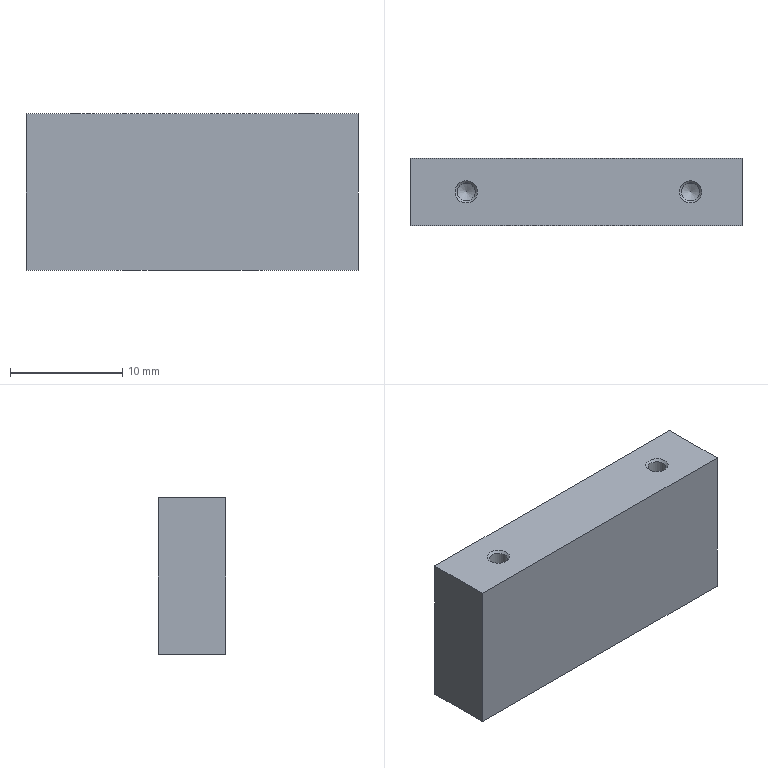Part | STEP file | Final stage amplifier press block | 1 solid | 18 faces | box 29.61 x 6 x 14 mm | volume 2437 mm3 | cone 8 | plane 6 | cylinder 4 | commonest cylinder face diameters 1.6 x4
STEP:
#1=CARTESIAN_POINT('',(0.,0.,0.));
#2=DIRECTION('',(0.,0.,1.));
#3=DIRECTION('',(1.,0.,0.));
#4=AXIS2_PLACEMENT_3D('',#1,#2,#3);
#5=CARTESIAN_POINT('',(-8.334,90.75,188.564));
#6=VERTEX_POINT('',#5);
#7=CARTESIAN_POINT('',(-8.334,84.75,188.564));
#8=VERTEX_POINT('',#7);
#9=CARTESIAN_POINT('',(-8.334,90.75,188.564));
#10=DIRECTION('',(0.,-1.,0.));
#11=VECTOR('',#10,1.);
#12=LINE('',#9,#11);
#13=CARTESIAN_POINT('',(-8.334,90.75,202.564));
#14=DIRECTION('',(1.,0.,0.));
#15=DIRECTION('',(0.,0.,-1.));
#16=AXIS2_PLACEMENT_3D('',#13,#14,#15);
#17=PLANE('',#16);
#18=CARTESIAN_POINT('',(14.,0.));
#19=DIRECTION('',(0.,-1.));
#20=VECTOR('',#19,1.);
#21=LINE('',#18,#20);
#22=(GEOMETRIC_REPRESENTATION_CONTEXT(2)PARAMETRIC_REPRESENTATION_CONTEXT()REPRESENTATION_CONTEXT('',''));
#23=DEFINITIONAL_REPRESENTATION('',(#21),#22);
#24=PCURVE('',#17,#23);
#25=CARTESIAN_POINT('',(0.,0.,188.564));
#26=DIRECTION('',(0.,0.,1.));
#27=DIRECTION('',(1.,0.,0.));
#28=AXIS2_PLACEMENT_3D('',#25,#26,#27);
#29=PLANE('',#28);
#30=CARTESIAN_POINT('',(-8.334,90.75));
#31=DIRECTION('',(0.,-1.));
#32=VECTOR('',#31,1.);
#33=LINE('',#30,#32);
#34=(GEOMETRIC_REPRESENTATION_CONTEXT(2)PARAMETRIC_REPRESENTATION_CONTEXT()REPRESENTATION_CONTEXT('',''));
#35=DEFINITIONAL_REPRESENTATION('',(#33),#34);
#36=PCURVE('',#29,#35);
#37=SURFACE_CURVE('',#12,(#24,#36),.PCURVE_S1.);
#38=EDGE_CURVE('',#6,#8,#37,.T.);
#39=ORIENTED_EDGE('',*,*,#38,.T.);
#40=CARTESIAN_POINT('',(-8.334,84.75,202.564));
#41=VERTEX_POINT('',#40);
#42=CARTESIAN_POINT('',(-8.334,84.75,202.564));
#43=DIRECTION('',(0.,0.,-1.));
#44=VECTOR('',#43,1.);
#45=LINE('',#42,#44);
#46=CARTESIAN_POINT('',(0.,-6.));
#47=DIRECTION('',(1.,0.));
#48=VECTOR('',#47,1.);
#49=LINE('',#46,#48);
#50=(GEOMETRIC_REPRESENTATION_CONTEXT(2)PARAMETRIC_REPRESENTATION_CONTEXT()REPRESENTATION_CONTEXT('',''));
#51=DEFINITIONAL_REPRESENTATION('',(#49),#50);
#52=PCURVE('',#17,#51);
#53=CARTESIAN_POINT('',(-8.334,84.75,202.564));
#54=DIRECTION('',(0.,1.,0.));
#55=DIRECTION('',(0.,0.,1.));
#56=AXIS2_PLACEMENT_3D('',#53,#54,#55);
#57=PLANE('',#56);
#58=CARTESIAN_POINT('',(0.,0.));
#59=DIRECTION('',(-1.,0.));
#60=VECTOR('',#59,1.);
#61=LINE('',#58,#60);
#62=(GEOMETRIC_REPRESENTATION_CONTEXT(2)PARAMETRIC_REPRESENTATION_CONTEXT()REPRESENTATION_CONTEXT('',''));
#63=DEFINITIONAL_REPRESENTATION('',(#61),#62);
#64=PCURVE('',#57,#63);
#65=SURFACE_CURVE('',#45,(#52,#64),.PCURVE_S1.);
#66=EDGE_CURVE('',#41,#8,#65,.T.);
#67=ORIENTED_EDGE('',*,*,#66,.F.);
#68=CARTESIAN_POINT('',(-8.334,90.75,202.564));
#69=VERTEX_POINT('',#68);
#70=CARTESIAN_POINT('',(-8.334,90.75,202.564));
#71=DIRECTION('',(0.,-1.,0.));
#72=VECTOR('',#71,1.);
#73=LINE('',#70,#72);
#74=CARTESIAN_POINT('',(0.,0.));
#75=DIRECTION('',(0.,-1.));
#76=VECTOR('',#75,1.);
#77=LINE('',#74,#76);
#78=(GEOMETRIC_REPRESENTATION_CONTEXT(2)PARAMETRIC_REPRESENTATION_CONTEXT()REPRESENTATION_CONTEXT('',''));
#79=DEFINITIONAL_REPRESENTATION('',(#77),#78);
#80=PCURVE('',#17,#79);
#81=CARTESIAN_POINT('',(0.,0.,202.564));
#82=DIRECTION('',(0.,0.,1.));
#83=DIRECTION('',(1.,0.,0.));
#84=AXIS2_PLACEMENT_3D('',#81,#82,#83);
#85=PLANE('',#84);
#86=CARTESIAN_POINT('',(-8.334,90.75));
#87=DIRECTION('',(0.,-1.));
#88=VECTOR('',#87,1.);
#89=LINE('',#86,#88);
#90=(GEOMETRIC_REPRESENTATION_CONTEXT(2)PARAMETRIC_REPRESENTATION_CONTEXT()REPRESENTATION_CONTEXT('',''));
#91=DEFINITIONAL_REPRESENTATION('',(#89),#90);
#92=PCURVE('',#85,#91);
#93=SURFACE_CURVE('',#73,(#80,#92),.PCURVE_S1.);
#94=EDGE_CURVE('',#69,#41,#93,.T.);
#95=ORIENTED_EDGE('',*,*,#94,.F.);
#96=CARTESIAN_POINT('',(-8.334,90.75,202.564));
#97=DIRECTION('',(0.,0.,-1.));
#98=VECTOR('',#97,1.);
#99=LINE('',#96,#98);
#100=CARTESIAN_POINT('',(0.,0.));
#101=DIRECTION('',(1.,0.));
#102=VECTOR('',#101,1.);
#103=LINE('',#100,#102);
#104=(GEOMETRIC_REPRESENTATION_CONTEXT(2)PARAMETRIC_REPRESENTATION_CONTEXT()REPRESENTATION_CONTEXT('',''));
#105=DEFINITIONAL_REPRESENTATION('',(#103),#104);
#106=PCURVE('',#17,#105);
#107=CARTESIAN_POINT('',(21.276,90.75,202.564));
#108=DIRECTION('',(0.,-1.,0.));
#109=DIRECTION('',(0.,0.,-1.));
#110=AXIS2_PLACEMENT_3D('',#107,#108,#109);
#111=PLANE('',#110);
#112=CARTESIAN_POINT('',(0.,-29.61));
#113=DIRECTION('',(1.,0.));
#114=VECTOR('',#113,1.);
#115=LINE('',#112,#114);
#116=(GEOMETRIC_REPRESENTATION_CONTEXT(2)PARAMETRIC_REPRESENTATION_CONTEXT()REPRESENTATION_CONTEXT('',''));
#117=DEFINITIONAL_REPRESENTATION('',(#115),#116);
#118=PCURVE('',#111,#117);
#119=SURFACE_CURVE('',#99,(#106,#118),.PCURVE_S1.);
#120=EDGE_CURVE('',#69,#6,#119,.T.);
#121=ORIENTED_EDGE('',*,*,#120,.T.);
#122=EDGE_LOOP('',(#39,#67,#95,#121));
#123=FACE_BOUND('',#122,.T.);
#124=ADVANCED_FACE('',(#123),#17,.F.);
#125=CARTESIAN_POINT('',(21.276,84.75,188.564));
#126=VERTEX_POINT('',#125);
#127=CARTESIAN_POINT('',(-8.334,84.75,188.564));
#128=DIRECTION('',(1.,0.,0.));
#129=VECTOR('',#128,1.);
#130=LINE('',#127,#129);
#131=CARTESIAN_POINT('',(-14.,0.));
#132=DIRECTION('',(0.,1.));
#133=VECTOR('',#132,1.);
#134=LINE('',#131,#133);
#135=(GEOMETRIC_REPRESENTATION_CONTEXT(2)PARAMETRIC_REPRESENTATION_CONTEXT()REPRESENTATION_CONTEXT('',''));
#136=DEFINITIONAL_REPRESENTATION('',(#134),#135);
#137=PCURVE('',#57,#136);
#138=CARTESIAN_POINT('',(-8.334,84.75));
#139=DIRECTION('',(1.,0.));
#140=VECTOR('',#139,1.);
#141=LINE('',#138,#140);
#142=(GEOMETRIC_REPRESENTATION_CONTEXT(2)PARAMETRIC_REPRESENTATION_CONTEXT()REPRESENTATION_CONTEXT('',''));
#143=DEFINITIONAL_REPRESENTATION('',(#141),#142);
#144=PCURVE('',#29,#143);
#145=SURFACE_CURVE('',#130,(#137,#144),.PCURVE_S1.);
#146=EDGE_CURVE('',#8,#126,#145,.T.);
#147=ORIENTED_EDGE('',*,*,#146,.T.);
#148=CARTESIAN_POINT('',(21.276,84.75,202.564));
#149=VERTEX_POINT('',#148);
#150=CARTESIAN_POINT('',(21.276,84.75,202.564));
#151=DIRECTION('',(0.,0.,-1.));
#152=VECTOR('',#151,1.);
#153=LINE('',#150,#152);
#154=CARTESIAN_POINT('',(0.,29.61));
#155=DIRECTION('',(-1.,0.));
#156=VECTOR('',#155,1.);
#157=LINE('',#154,#156);
#158=(GEOMETRIC_REPRESENTATION_CONTEXT(2)PARAMETRIC_REPRESENTATION_CONTEXT()REPRESENTATION_CONTEXT('',''));
#159=DEFINITIONAL_REPRESENTATION('',(#157),#158);
#160=PCURVE('',#57,#159);
#161=CARTESIAN_POINT('',(21.276,84.75,202.564));
#162=DIRECTION('',(-1.,0.,0.));
#163=DIRECTION('',(0.,0.,1.));
#164=AXIS2_PLACEMENT_3D('',#161,#162,#163);
#165=PLANE('',#164);
#166=CARTESIAN_POINT('',(0.,0.));
#167=DIRECTION('',(-1.,0.));
#168=VECTOR('',#167,1.);
#169=LINE('',#166,#168);
#170=(GEOMETRIC_REPRESENTATION_CONTEXT(2)PARAMETRIC_REPRESENTATION_CONTEXT()REPRESENTATION_CONTEXT('',''));
#171=DEFINITIONAL_REPRESENTATION('',(#169),#170);
#172=PCURVE('',#165,#171);
#173=SURFACE_CURVE('',#153,(#160,#172),.PCURVE_S1.);
#174=EDGE_CURVE('',#149,#126,#173,.T.);
#175=ORIENTED_EDGE('',*,*,#174,.F.);
#176=CARTESIAN_POINT('',(-8.334,84.75,202.564));
#177=DIRECTION('',(1.,0.,0.));
#178=VECTOR('',#177,1.);
#179=LINE('',#176,#178);
#180=CARTESIAN_POINT('',(0.,0.));
#181=DIRECTION('',(0.,1.));
#182=VECTOR('',#181,1.);
#183=LINE('',#180,#182);
#184=(GEOMETRIC_REPRESENTATION_CONTEXT(2)PARAMETRIC_REPRESENTATION_CONTEXT()REPRESENTATION_CONTEXT('',''));
#185=DEFINITIONAL_REPRESENTATION('',(#183),#184);
#186=PCURVE('',#57,#185);
#187=CARTESIAN_POINT('',(-8.334,84.75));
#188=DIRECTION('',(1.,0.));
#189=VECTOR('',#188,1.);
#190=LINE('',#187,#189);
#191=(GEOMETRIC_REPRESENTATION_CONTEXT(2)PARAMETRIC_REPRESENTATION_CONTEXT()REPRESENTATION_CONTEXT('',''));
#192=DEFINITIONAL_REPRESENTATION('',(#190),#191);
#193=PCURVE('',#85,#192);
#194=SURFACE_CURVE('',#179,(#186,#193),.PCURVE_S1.);
#195=EDGE_CURVE('',#41,#149,#194,.T.);
#196=ORIENTED_EDGE('',*,*,#195,.F.);
#197=ORIENTED_EDGE('',*,*,#66,.T.);
#198=EDGE_LOOP('',(#147,#175,#196,#197));
#199=FACE_BOUND('',#198,.T.);
#200=ADVANCED_FACE('',(#199),#57,.F.);
#201=CARTESIAN_POINT('',(21.276,90.75,188.564));
#202=VERTEX_POINT('',#201);
#203=CARTESIAN_POINT('',(21.276,84.75,188.564));
#204=DIRECTION('',(0.,1.,0.));
#205=VECTOR('',#204,1.);
#206=LINE('',#203,#205);
#207=CARTESIAN_POINT('',(-14.,0.));
#208=DIRECTION('',(0.,1.));
#209=VECTOR('',#208,1.);
#210=LINE('',#207,#209);
#211=(GEOMETRIC_REPRESENTATION_CONTEXT(2)PARAMETRIC_REPRESENTATION_CONTEXT()REPRESENTATION_CONTEXT('',''));
#212=DEFINITIONAL_REPRESENTATION('',(#210),#211);
#213=PCURVE('',#165,#212);
#214=CARTESIAN_POINT('',(21.276,84.75));
#215=DIRECTION('',(0.,1.));
#216=VECTOR('',#215,1.);
#217=LINE('',#214,#216);
#218=(GEOMETRIC_REPRESENTATION_CONTEXT(2)PARAMETRIC_REPRESENTATION_CONTEXT()REPRESENTATION_CONTEXT('',''));
#219=DEFINITIONAL_REPRESENTATION('',(#217),#218);
#220=PCURVE('',#29,#219);
#221=SURFACE_CURVE('',#206,(#213,#220),.PCURVE_S1.);
#222=EDGE_CURVE('',#126,#202,#221,.T.);
#223=ORIENTED_EDGE('',*,*,#222,.T.);
#224=CARTESIAN_POINT('',(21.276,90.75,202.564));
#225=VERTEX_POINT('',#224);
#226=CARTESIAN_POINT('',(21.276,90.75,202.564));
#227=DIRECTION('',(0.,0.,-1.));
#228=VECTOR('',#227,1.);
#229=LINE('',#226,#228);
#230=CARTESIAN_POINT('',(0.,6.));
#231=DIRECTION('',(-1.,0.));
#232=VECTOR('',#231,1.);
#233=LINE('',#230,#232);
#234=(GEOMETRIC_REPRESENTATION_CONTEXT(2)PARAMETRIC_REPRESENTATION_CONTEXT()REPRESENTATION_CONTEXT('',''));
#235=DEFINITIONAL_REPRESENTATION('',(#233),#234);
#236=PCURVE('',#165,#235);
#237=CARTESIAN_POINT('',(0.,0.));
#238=DIRECTION('',(1.,0.));
#239=VECTOR('',#238,1.);
#240=LINE('',#237,#239);
#241=(GEOMETRIC_REPRESENTATION_CONTEXT(2)PARAMETRIC_REPRESENTATION_CONTEXT()REPRESENTATION_CONTEXT('',''));
#242=DEFINITIONAL_REPRESENTATION('',(#240),#241);
#243=PCURVE('',#111,#242);
#244=SURFACE_CURVE('',#229,(#236,#243),.PCURVE_S1.);
#245=EDGE_CURVE('',#225,#202,#244,.T.);
#246=ORIENTED_EDGE('',*,*,#245,.F.);
#247=CARTESIAN_POINT('',(21.276,84.75,202.564));
#248=DIRECTION('',(0.,1.,0.));
#249=VECTOR('',#248,1.);
#250=LINE('',#247,#249);
#251=CARTESIAN_POINT('',(0.,0.));
#252=DIRECTION('',(0.,1.));
#253=VECTOR('',#252,1.);
#254=LINE('',#251,#253);
#255=(GEOMETRIC_REPRESENTATION_CONTEXT(2)PARAMETRIC_REPRESENTATION_CONTEXT()REPRESENTATION_CONTEXT('',''));
#256=DEFINITIONAL_REPRESENTATION('',(#254),#255);
#257=PCURVE('',#165,#256);
#258=CARTESIAN_POINT('',(21.276,84.75));
#259=DIRECTION('',(0.,1.));
#260=VECTOR('',#259,1.);
#261=LINE('',#258,#260);
#262=(GEOMETRIC_REPRESENTATION_CONTEXT(2)PARAMETRIC_REPRESENTATION_CONTEXT()REPRESENTATION_CONTEXT('',''));
#263=DEFINITIONAL_REPRESENTATION('',(#261),#262);
#264=PCURVE('',#85,#263);
#265=SURFACE_CURVE('',#250,(#257,#264),.PCURVE_S1.);
#266=EDGE_CURVE('',#149,#225,#265,.T.);
#267=ORIENTED_EDGE('',*,*,#266,.F.);
#268=ORIENTED_EDGE('',*,*,#174,.T.);
#269=EDGE_LOOP('',(#223,#246,#267,#268));
#270=FACE_BOUND('',#269,.T.);
#271=ADVANCED_FACE('',(#270),#165,.F.);
#272=CARTESIAN_POINT('',(21.276,90.75,188.564));
#273=DIRECTION('',(-1.,0.,0.));
#274=VECTOR('',#273,1.);
#275=LINE('',#272,#274);
#276=CARTESIAN_POINT('',(14.,0.));
#277=DIRECTION('',(0.,-1.));
#278=VECTOR('',#277,1.);
#279=LINE('',#276,#278);
#280=(GEOMETRIC_REPRESENTATION_CONTEXT(2)PARAMETRIC_REPRESENTATION_CONTEXT()REPRESENTATION_CONTEXT('',''));
#281=DEFINITIONAL_REPRESENTATION('',(#279),#280);
#282=PCURVE('',#111,#281);
#283=CARTESIAN_POINT('',(21.276,90.75));
#284=DIRECTION('',(-1.,0.));
#285=VECTOR('',#284,1.);
#286=LINE('',#283,#285);
#287=(GEOMETRIC_REPRESENTATION_CONTEXT(2)PARAMETRIC_REPRESENTATION_CONTEXT()REPRESENTATION_CONTEXT('',''));
#288=DEFINITIONAL_REPRESENTATION('',(#286),#287);
#289=PCURVE('',#29,#288);
#290=SURFACE_CURVE('',#275,(#282,#289),.PCURVE_S1.);
#291=EDGE_CURVE('',#202,#6,#290,.T.);
#292=ORIENTED_EDGE('',*,*,#291,.T.);
#293=ORIENTED_EDGE('',*,*,#120,.F.);
#294=CARTESIAN_POINT('',(21.276,90.75,202.564));
#295=DIRECTION('',(-1.,0.,0.));
#296=VECTOR('',#295,1.);
#297=LINE('',#294,#296);
#298=CARTESIAN_POINT('',(0.,0.));
#299=DIRECTION('',(0.,-1.));
#300=VECTOR('',#299,1.);
#301=LINE('',#298,#300);
#302=(GEOMETRIC_REPRESENTATION_CONTEXT(2)PARAMETRIC_REPRESENTATION_CONTEXT()REPRESENTATION_CONTEXT('',''));
#303=DEFINITIONAL_REPRESENTATION('',(#301),#302);
#304=PCURVE('',#111,#303);
#305=CARTESIAN_POINT('',(21.276,90.75));
#306=DIRECTION('',(-1.,0.));
#307=VECTOR('',#306,1.);
#308=LINE('',#305,#307);
#309=(GEOMETRIC_REPRESENTATION_CONTEXT(2)PARAMETRIC_REPRESENTATION_CONTEXT()REPRESENTATION_CONTEXT('',''));
#310=DEFINITIONAL_REPRESENTATION('',(#308),#309);
#311=PCURVE('',#85,#310);
#312=SURFACE_CURVE('',#297,(#304,#311),.PCURVE_S1.);
#313=EDGE_CURVE('',#225,#69,#312,.T.);
#314=ORIENTED_EDGE('',*,*,#313,.F.);
#315=ORIENTED_EDGE('',*,*,#245,.T.);
#316=EDGE_LOOP('',(#292,#293,#314,#315));
#317=FACE_BOUND('',#316,.T.);
#318=ADVANCED_FACE('',(#317),#111,.F.);
#319=CARTESIAN_POINT('',(17.682,87.75,202.564));
#320=VERTEX_POINT('',#319);
#321=CARTESIAN_POINT('',(16.682,87.75,202.564));
#322=DIRECTION('',(0.,0.,1.));
#323=DIRECTION('',(1.,0.,0.));
#324=AXIS2_PLACEMENT_3D('',#321,#322,#323);
#325=CIRCLE('',#324,1.);
#326=CARTESIAN_POINT('',(16.682,87.75));
#327=DIRECTION('',(1.,0.));
#328=AXIS2_PLACEMENT_2D('',#326,#327);
#329=CIRCLE('',#328,1.);
#330=(GEOMETRIC_REPRESENTATION_CONTEXT(2)PARAMETRIC_REPRESENTATION_CONTEXT()REPRESENTATION_CONTEXT('',''));
#331=DEFINITIONAL_REPRESENTATION('',(#329),#330);
#332=PCURVE('',#85,#331);
#333=CARTESIAN_POINT('',(16.682,87.75,201.564));
#334=DIRECTION('',(0.,0.,1.));
#335=DIRECTION('',(1.,0.,0.));
#336=AXIS2_PLACEMENT_3D('',#333,#334,#335);
#337=CONICAL_SURFACE('',#336,0.,0.7854);
#338=CARTESIAN_POINT('',(0.,1.));
#339=DIRECTION('',(1.,0.));
#340=VECTOR('',#339,1.);
#341=LINE('',#338,#340);
#342=(GEOMETRIC_REPRESENTATION_CONTEXT(2)PARAMETRIC_REPRESENTATION_CONTEXT()REPRESENTATION_CONTEXT('',''));
#343=DEFINITIONAL_REPRESENTATION('',(#341),#342);
#344=PCURVE('',#337,#343);
#345=SURFACE_CURVE('',#325,(#332,#344),.PCURVE_S1.);
#346=EDGE_CURVE('',#320,#320,#345,.T.);
#347=ORIENTED_EDGE('',*,*,#346,.F.);
#348=EDGE_LOOP('',(#347));
#349=FACE_BOUND('',#348,.T.);
#350=CARTESIAN_POINT('',(-2.318,87.75,202.564));
#351=VERTEX_POINT('',#350);
#352=CARTESIAN_POINT('',(-3.318,87.75,202.564));
#353=DIRECTION('',(0.,0.,1.));
#354=DIRECTION('',(1.,0.,0.));
#355=AXIS2_PLACEMENT_3D('',#352,#353,#354);
#356=CIRCLE('',#355,1.);
#357=CARTESIAN_POINT('',(-3.318,87.75));
#358=DIRECTION('',(1.,0.));
#359=AXIS2_PLACEMENT_2D('',#357,#358);
#360=CIRCLE('',#359,1.);
#361=(GEOMETRIC_REPRESENTATION_CONTEXT(2)PARAMETRIC_REPRESENTATION_CONTEXT()REPRESENTATION_CONTEXT('',''));
#362=DEFINITIONAL_REPRESENTATION('',(#360),#361);
#363=PCURVE('',#85,#362);
#364=CARTESIAN_POINT('',(-3.318,87.75,201.564));
#365=DIRECTION('',(0.,0.,1.));
#366=DIRECTION('',(1.,0.,0.));
#367=AXIS2_PLACEMENT_3D('',#364,#365,#366);
#368=CONICAL_SURFACE('',#367,0.,0.7854);
#369=CARTESIAN_POINT('',(0.,1.));
#370=DIRECTION('',(1.,0.));
#371=VECTOR('',#370,1.);
#372=LINE('',#369,#371);
#373=(GEOMETRIC_REPRESENTATION_CONTEXT(2)PARAMETRIC_REPRESENTATION_CONTEXT()REPRESENTATION_CONTEXT('',''));
#374=DEFINITIONAL_REPRESENTATION('',(#372),#373);
#375=PCURVE('',#368,#374);
#376=SURFACE_CURVE('',#356,(#363,#375),.PCURVE_S1.);
#377=EDGE_CURVE('',#351,#351,#376,.T.);
#378=ORIENTED_EDGE('',*,*,#377,.F.);
#379=EDGE_LOOP('',(#378));
#380=FACE_BOUND('',#379,.T.);
#381=ORIENTED_EDGE('',*,*,#94,.T.);
#382=ORIENTED_EDGE('',*,*,#195,.T.);
#383=ORIENTED_EDGE('',*,*,#266,.T.);
#384=ORIENTED_EDGE('',*,*,#313,.T.);
#385=EDGE_LOOP('',(#381,#382,#383,#384));
#386=FACE_BOUND('',#385,.T.);
#387=ADVANCED_FACE('',(#349,#380,#386),#85,.T.);
#388=CARTESIAN_POINT('',(12.682,87.58,188.564));
#389=VERTEX_POINT('',#388);
#390=CARTESIAN_POINT('',(10.682,87.58,188.564));
#391=VERTEX_POINT('',#390);
#392=CARTESIAN_POINT('',(11.682,87.58,188.564));
#393=DIRECTION('',(0.,0.,1.));
#394=DIRECTION('',(1.,0.,0.));
#395=AXIS2_PLACEMENT_3D('',#392,#393,#394);
#396=CIRCLE('',#395,1.);
#397=CARTESIAN_POINT('',(11.682,87.58));
#398=DIRECTION('',(1.,0.));
#399=AXIS2_PLACEMENT_2D('',#397,#398);
#400=CIRCLE('',#399,1.);
#401=(GEOMETRIC_REPRESENTATION_CONTEXT(2)PARAMETRIC_REPRESENTATION_CONTEXT()REPRESENTATION_CONTEXT('',''));
#402=DEFINITIONAL_REPRESENTATION('',(#400),#401);
#403=PCURVE('',#29,#402);
#404=CARTESIAN_POINT('',(11.682,87.58,189.564));
#405=DIRECTION('',(0.,0.,-1.));
#406=DIRECTION('',(-1.,0.,0.));
#407=AXIS2_PLACEMENT_3D('',#404,#405,#406);
#408=CONICAL_SURFACE('',#407,0.,0.7854);
#409=CARTESIAN_POINT('',(3.142,1.));
#410=DIRECTION('',(-1.,0.));
#411=VECTOR('',#410,1.);
#412=LINE('',#409,#411);
#413=(GEOMETRIC_REPRESENTATION_CONTEXT(2)PARAMETRIC_REPRESENTATION_CONTEXT()REPRESENTATION_CONTEXT('',''));
#414=DEFINITIONAL_REPRESENTATION('',(#412),#413);
#415=PCURVE('',#408,#414);
#416=SURFACE_CURVE('',#396,(#403,#415),.PCURVE_S1.);
#417=EDGE_CURVE('',#389,#391,#416,.T.);
#418=ORIENTED_EDGE('',*,*,#417,.T.);
#419=CARTESIAN_POINT('',(11.682,87.58,188.564));
#420=DIRECTION('',(0.,0.,1.));
#421=DIRECTION('',(1.,0.,0.));
#422=AXIS2_PLACEMENT_3D('',#419,#420,#421);
#423=CIRCLE('',#422,1.);
#424=CARTESIAN_POINT('',(11.682,87.58));
#425=DIRECTION('',(1.,0.));
#426=AXIS2_PLACEMENT_2D('',#424,#425);
#427=CIRCLE('',#426,1.);
#428=(GEOMETRIC_REPRESENTATION_CONTEXT(2)PARAMETRIC_REPRESENTATION_CONTEXT()REPRESENTATION_CONTEXT('',''));
#429=DEFINITIONAL_REPRESENTATION('',(#427),#428);
#430=PCURVE('',#29,#429);
#431=CARTESIAN_POINT('',(9.425,1.));
#432=DIRECTION('',(-1.,0.));
#433=VECTOR('',#432,1.);
#434=LINE('',#431,#433);
#435=(GEOMETRIC_REPRESENTATION_CONTEXT(2)PARAMETRIC_REPRESENTATION_CONTEXT()REPRESENTATION_CONTEXT('',''));
#436=DEFINITIONAL_REPRESENTATION('',(#434),#435);
#437=PCURVE('',#408,#436);
#438=SURFACE_CURVE('',#423,(#430,#437),.PCURVE_S1.);
#439=EDGE_CURVE('',#391,#389,#438,.T.);
#440=ORIENTED_EDGE('',*,*,#439,.T.);
#441=EDGE_LOOP('',(#418,#440));
#442=FACE_BOUND('',#441,.T.);
#443=CARTESIAN_POINT('',(2.682,87.58,188.564));
#444=VERTEX_POINT('',#443);
#445=CARTESIAN_POINT('',(0.6818,87.58,188.564));
#446=VERTEX_POINT('',#445);
#447=CARTESIAN_POINT('',(1.682,87.58,188.564));
#448=DIRECTION('',(0.,0.,1.));
#449=DIRECTION('',(1.,0.,0.));
#450=AXIS2_PLACEMENT_3D('',#447,#448,#449);
#451=CIRCLE('',#450,1.);
#452=CARTESIAN_POINT('',(1.682,87.58));
#453=DIRECTION('',(1.,0.));
#454=AXIS2_PLACEMENT_2D('',#452,#453);
#455=CIRCLE('',#454,1.);
#456=(GEOMETRIC_REPRESENTATION_CONTEXT(2)PARAMETRIC_REPRESENTATION_CONTEXT()REPRESENTATION_CONTEXT('',''));
#457=DEFINITIONAL_REPRESENTATION('',(#455),#456);
#458=PCURVE('',#29,#457);
#459=CARTESIAN_POINT('',(1.682,87.58,189.564));
#460=DIRECTION('',(0.,0.,-1.));
#461=DIRECTION('',(-1.,0.,0.));
#462=AXIS2_PLACEMENT_3D('',#459,#460,#461);
#463=CONICAL_SURFACE('',#462,0.,0.7854);
#464=CARTESIAN_POINT('',(3.142,1.));
#465=DIRECTION('',(-1.,0.));
#466=VECTOR('',#465,1.);
#467=LINE('',#464,#466);
#468=(GEOMETRIC_REPRESENTATION_CONTEXT(2)PARAMETRIC_REPRESENTATION_CONTEXT()REPRESENTATION_CONTEXT('',''));
#469=DEFINITIONAL_REPRESENTATION('',(#467),#468);
#470=PCURVE('',#463,#469);
#471=SURFACE_CURVE('',#451,(#458,#470),.PCURVE_S1.);
#472=EDGE_CURVE('',#444,#446,#471,.T.);
#473=ORIENTED_EDGE('',*,*,#472,.T.);
#474=CARTESIAN_POINT('',(1.682,87.58,188.564));
#475=DIRECTION('',(0.,0.,1.));
#476=DIRECTION('',(1.,0.,0.));
#477=AXIS2_PLACEMENT_3D('',#474,#475,#476);
#478=CIRCLE('',#477,1.);
#479=CARTESIAN_POINT('',(1.682,87.58));
#480=DIRECTION('',(1.,0.));
#481=AXIS2_PLACEMENT_2D('',#479,#480);
#482=CIRCLE('',#481,1.);
#483=(GEOMETRIC_REPRESENTATION_CONTEXT(2)PARAMETRIC_REPRESENTATION_CONTEXT()REPRESENTATION_CONTEXT('',''));
#484=DEFINITIONAL_REPRESENTATION('',(#482),#483);
#485=PCURVE('',#29,#484);
#486=CARTESIAN_POINT('',(9.425,1.));
#487=DIRECTION('',(-1.,0.));
#488=VECTOR('',#487,1.);
#489=LINE('',#486,#488);
#490=(GEOMETRIC_REPRESENTATION_CONTEXT(2)PARAMETRIC_REPRESENTATION_CONTEXT()REPRESENTATION_CONTEXT('',''));
#491=DEFINITIONAL_REPRESENTATION('',(#489),#490);
#492=PCURVE('',#463,#491);
#493=SURFACE_CURVE('',#478,(#485,#492),.PCURVE_S1.);
#494=EDGE_CURVE('',#446,#444,#493,.T.);
#495=ORIENTED_EDGE('',*,*,#494,.T.);
#496=EDGE_LOOP('',(#473,#495));
#497=FACE_BOUND('',#496,.T.);
#498=ORIENTED_EDGE('',*,*,#38,.F.);
#499=ORIENTED_EDGE('',*,*,#291,.F.);
#500=ORIENTED_EDGE('',*,*,#222,.F.);
#501=ORIENTED_EDGE('',*,*,#146,.F.);
#502=EDGE_LOOP('',(#498,#499,#500,#501));
#503=FACE_BOUND('',#502,.T.);
#504=ADVANCED_FACE('',(#442,#497,#503),#29,.F.);
#505=ORIENTED_EDGE('',*,*,#377,.F.);
#506=CARTESIAN_POINT('',(-2.518,87.75,202.364));
#507=VERTEX_POINT('',#506);
#508=CARTESIAN_POINT('',(-2.518,87.75,202.364));
#509=CARTESIAN_POINT('',(-2.318,87.75,202.564));
#510=B_SPLINE_CURVE_WITH_KNOTS('',1,(#508,#509),.UNSPECIFIED.,.F.,.F.,(2,2),(1.131,1.414),.PIECEWISE_BEZIER_KNOTS.);
#511=CARTESIAN_POINT('',(0.,0.));
#512=DIRECTION('',(0.,1.));
#513=VECTOR('',#512,1.);
#514=LINE('',#511,#513);
#515=(GEOMETRIC_REPRESENTATION_CONTEXT(2)PARAMETRIC_REPRESENTATION_CONTEXT()REPRESENTATION_CONTEXT('',''));
#516=DEFINITIONAL_REPRESENTATION('',(#514),#515);
#517=PCURVE('',#368,#516);
#518=CARTESIAN_POINT('',(6.283,0.));
#519=DIRECTION('',(0.,1.));
#520=VECTOR('',#519,1.);
#521=LINE('',#518,#520);
#522=(GEOMETRIC_REPRESENTATION_CONTEXT(2)PARAMETRIC_REPRESENTATION_CONTEXT()REPRESENTATION_CONTEXT('',''));
#523=DEFINITIONAL_REPRESENTATION('',(#521),#522);
#524=PCURVE('',#368,#523);
#525=SEAM_CURVE('',#510,(#517,#524),.PCURVE_S1.);
#526=EDGE_CURVE('',#507,#351,#525,.T.);
#527=ORIENTED_EDGE('',*,*,#526,.F.);
#528=CARTESIAN_POINT('',(-3.318,87.75,202.364));
#529=DIRECTION('',(0.,0.,1.));
#530=DIRECTION('',(1.,0.,0.));
#531=AXIS2_PLACEMENT_3D('',#528,#529,#530);
#532=CIRCLE('',#531,0.8);
#533=CARTESIAN_POINT('',(0.,0.8));
#534=DIRECTION('',(1.,0.));
#535=VECTOR('',#534,1.);
#536=LINE('',#533,#535);
#537=(GEOMETRIC_REPRESENTATION_CONTEXT(2)PARAMETRIC_REPRESENTATION_CONTEXT()REPRESENTATION_CONTEXT('',''));
#538=DEFINITIONAL_REPRESENTATION('',(#536),#537);
#539=PCURVE('',#368,#538);
#540=CARTESIAN_POINT('',(-3.318,87.75,202.564));
#541=DIRECTION('',(0.,0.,-1.));
#542=DIRECTION('',(-1.,0.,0.));
#543=AXIS2_PLACEMENT_3D('',#540,#541,#542);
#544=CYLINDRICAL_SURFACE('',#543,0.8);
#545=CARTESIAN_POINT('',(9.425,0.2));
#546=DIRECTION('',(-1.,0.));
#547=VECTOR('',#546,1.);
#548=LINE('',#545,#547);
#549=(GEOMETRIC_REPRESENTATION_CONTEXT(2)PARAMETRIC_REPRESENTATION_CONTEXT()REPRESENTATION_CONTEXT('',''));
#550=DEFINITIONAL_REPRESENTATION('',(#548),#549);
#551=PCURVE('',#544,#550);
#552=SURFACE_CURVE('',#532,(#539,#551),.PCURVE_S1.);
#553=EDGE_CURVE('',#507,#507,#552,.T.);
#554=ORIENTED_EDGE('',*,*,#553,.T.);
#555=ORIENTED_EDGE('',*,*,#526,.T.);
#556=EDGE_LOOP('',(#505,#527,#554,#555));
#557=FACE_BOUND('',#556,.F.);
#558=ADVANCED_FACE('',(#557),#368,.F.);
#559=CARTESIAN_POINT('',(-2.518,87.75,196.564));
#560=VERTEX_POINT('',#559);
#561=CARTESIAN_POINT('',(-4.118,87.75,196.564));
#562=VERTEX_POINT('',#561);
#563=CARTESIAN_POINT('',(-3.318,87.75,196.564));
#564=DIRECTION('',(0.,0.,1.));
#565=DIRECTION('',(-1.,0.,0.));
#566=AXIS2_PLACEMENT_3D('',#563,#564,#565);
#567=CIRCLE('',#566,0.8);
#568=CARTESIAN_POINT('',(-3.318,87.75,196.564));
#569=DIRECTION('',(0.,0.,1.));
#570=DIRECTION('',(1.,0.,0.));
#571=AXIS2_PLACEMENT_3D('',#568,#569,#570);
#572=CONICAL_SURFACE('',#571,0.8,1.03);
#573=CARTESIAN_POINT('',(-3.142,0.));
#574=DIRECTION('',(1.,0.));
#575=VECTOR('',#574,1.);
#576=LINE('',#573,#575);
#577=(GEOMETRIC_REPRESENTATION_CONTEXT(2)PARAMETRIC_REPRESENTATION_CONTEXT()REPRESENTATION_CONTEXT('',''));
#578=DEFINITIONAL_REPRESENTATION('',(#576),#577);
#579=PCURVE('',#572,#578);
#580=CARTESIAN_POINT('',(12.566,6.));
#581=DIRECTION('',(-1.,0.));
#582=VECTOR('',#581,1.);
#583=LINE('',#580,#582);
#584=(GEOMETRIC_REPRESENTATION_CONTEXT(2)PARAMETRIC_REPRESENTATION_CONTEXT()REPRESENTATION_CONTEXT('',''));
#585=DEFINITIONAL_REPRESENTATION('',(#583),#584);
#586=PCURVE('',#544,#585);
#587=SURFACE_CURVE('',#567,(#579,#586),.PCURVE_S1.);
#588=EDGE_CURVE('',#560,#562,#587,.T.);
#589=ORIENTED_EDGE('',*,*,#588,.F.);
#590=CARTESIAN_POINT('',(-3.318,87.75,196.083));
#591=VERTEX_POINT('',#590);
#592=CARTESIAN_POINT('',(-3.318,87.75,196.083));
#593=CARTESIAN_POINT('',(-2.518,87.75,196.564));
#594=B_SPLINE_CURVE_WITH_KNOTS('',1,(#592,#593),.UNSPECIFIED.,.F.,.F.,(2,2),(-0.9333,0.),.PIECEWISE_BEZIER_KNOTS.);
#595=CARTESIAN_POINT('',(0.,0.));
#596=DIRECTION('',(0.,1.));
#597=VECTOR('',#596,1.);
#598=LINE('',#595,#597);
#599=(GEOMETRIC_REPRESENTATION_CONTEXT(2)PARAMETRIC_REPRESENTATION_CONTEXT()REPRESENTATION_CONTEXT('',''));
#600=DEFINITIONAL_REPRESENTATION('',(#598),#599);
#601=PCURVE('',#572,#600);
#602=CARTESIAN_POINT('',(6.283,0.));
#603=DIRECTION('',(0.,1.));
#604=VECTOR('',#603,1.);
#605=LINE('',#602,#604);
#606=(GEOMETRIC_REPRESENTATION_CONTEXT(2)PARAMETRIC_REPRESENTATION_CONTEXT()REPRESENTATION_CONTEXT('',''));
#607=DEFINITIONAL_REPRESENTATION('',(#605),#606);
#608=PCURVE('',#572,#607);
#609=SEAM_CURVE('',#594,(#601,#608),.PCURVE_S1.);
#610=EDGE_CURVE('',#591,#560,#609,.T.);
#611=ORIENTED_EDGE('',*,*,#610,.F.);
#612=ORIENTED_EDGE('',*,*,#610,.T.);
#613=CARTESIAN_POINT('',(-3.318,87.75,196.564));
#614=DIRECTION('',(0.,0.,1.));
#615=DIRECTION('',(-1.,0.,0.));
#616=AXIS2_PLACEMENT_3D('',#613,#614,#615);
#617=CIRCLE('',#616,0.8);
#618=CARTESIAN_POINT('',(3.142,0.));
#619=DIRECTION('',(1.,0.));
#620=VECTOR('',#619,1.);
#621=LINE('',#618,#620);
#622=(GEOMETRIC_REPRESENTATION_CONTEXT(2)PARAMETRIC_REPRESENTATION_CONTEXT()REPRESENTATION_CONTEXT('',''));
#623=DEFINITIONAL_REPRESENTATION('',(#621),#622);
#624=PCURVE('',#572,#623);
#625=CARTESIAN_POINT('',(6.283,6.));
#626=DIRECTION('',(-1.,0.));
#627=VECTOR('',#626,1.);
#628=LINE('',#625,#627);
#629=(GEOMETRIC_REPRESENTATION_CONTEXT(2)PARAMETRIC_REPRESENTATION_CONTEXT()REPRESENTATION_CONTEXT('',''));
#630=DEFINITIONAL_REPRESENTATION('',(#628),#629);
#631=PCURVE('',#544,#630);
#632=SURFACE_CURVE('',#617,(#624,#631),.PCURVE_S1.);
#633=EDGE_CURVE('',#562,#560,#632,.T.);
#634=ORIENTED_EDGE('',*,*,#633,.F.);
#635=EDGE_LOOP('',(#589,#611,#612,#634));
#636=FACE_BOUND('',#635,.F.);
#637=ADVANCED_FACE('',(#636),#572,.F.);
#638=ORIENTED_EDGE('',*,*,#553,.F.);
#639=CARTESIAN_POINT('',(-2.518,87.75,202.364));
#640=CARTESIAN_POINT('',(-2.518,87.75,196.564));
#641=B_SPLINE_CURVE_WITH_KNOTS('',1,(#639,#640),.UNSPECIFIED.,.F.,.F.,(2,2),(0.2,6.),.PIECEWISE_BEZIER_KNOTS.);
#642=CARTESIAN_POINT('',(9.425,0.));
#643=DIRECTION('',(0.,1.));
#644=VECTOR('',#643,1.);
#645=LINE('',#642,#644);
#646=(GEOMETRIC_REPRESENTATION_CONTEXT(2)PARAMETRIC_REPRESENTATION_CONTEXT()REPRESENTATION_CONTEXT('',''));
#647=DEFINITIONAL_REPRESENTATION('',(#645),#646);
#648=PCURVE('',#544,#647);
#649=CARTESIAN_POINT('',(3.142,0.));
#650=DIRECTION('',(0.,1.));
#651=VECTOR('',#650,1.);
#652=LINE('',#649,#651);
#653=(GEOMETRIC_REPRESENTATION_CONTEXT(2)PARAMETRIC_REPRESENTATION_CONTEXT()REPRESENTATION_CONTEXT('',''));
#654=DEFINITIONAL_REPRESENTATION('',(#652),#653);
#655=PCURVE('',#544,#654);
#656=SEAM_CURVE('',#641,(#648,#655),.PCURVE_S1.);
#657=EDGE_CURVE('',#507,#560,#656,.T.);
#658=ORIENTED_EDGE('',*,*,#657,.T.);
#659=ORIENTED_EDGE('',*,*,#588,.T.);
#660=ORIENTED_EDGE('',*,*,#633,.T.);
#661=ORIENTED_EDGE('',*,*,#657,.F.);
#662=EDGE_LOOP('',(#638,#658,#659,#660,#661));
#663=FACE_BOUND('',#662,.F.);
#664=ADVANCED_FACE('',(#663),#544,.F.);
#665=ORIENTED_EDGE('',*,*,#346,.F.);
#666=CARTESIAN_POINT('',(17.482,87.75,202.364));
#667=VERTEX_POINT('',#666);
#668=CARTESIAN_POINT('',(17.482,87.75,202.364));
#669=CARTESIAN_POINT('',(17.682,87.75,202.564));
#670=B_SPLINE_CURVE_WITH_KNOTS('',1,(#668,#669),.UNSPECIFIED.,.F.,.F.,(2,2),(1.131,1.414),.PIECEWISE_BEZIER_KNOTS.);
#671=CARTESIAN_POINT('',(0.,0.));
#672=DIRECTION('',(0.,1.));
#673=VECTOR('',#672,1.);
#674=LINE('',#671,#673);
#675=(GEOMETRIC_REPRESENTATION_CONTEXT(2)PARAMETRIC_REPRESENTATION_CONTEXT()REPRESENTATION_CONTEXT('',''));
#676=DEFINITIONAL_REPRESENTATION('',(#674),#675);
#677=PCURVE('',#337,#676);
#678=CARTESIAN_POINT('',(6.283,0.));
#679=DIRECTION('',(0.,1.));
#680=VECTOR('',#679,1.);
#681=LINE('',#678,#680);
#682=(GEOMETRIC_REPRESENTATION_CONTEXT(2)PARAMETRIC_REPRESENTATION_CONTEXT()REPRESENTATION_CONTEXT('',''));
#683=DEFINITIONAL_REPRESENTATION('',(#681),#682);
#684=PCURVE('',#337,#683);
#685=SEAM_CURVE('',#670,(#677,#684),.PCURVE_S1.);
#686=EDGE_CURVE('',#667,#320,#685,.T.);
#687=ORIENTED_EDGE('',*,*,#686,.F.);
#688=CARTESIAN_POINT('',(16.682,87.75,202.364));
#689=DIRECTION('',(0.,0.,1.));
#690=DIRECTION('',(1.,0.,0.));
#691=AXIS2_PLACEMENT_3D('',#688,#689,#690);
#692=CIRCLE('',#691,0.8);
#693=CARTESIAN_POINT('',(0.,0.8));
#694=DIRECTION('',(1.,0.));
#695=VECTOR('',#694,1.);
#696=LINE('',#693,#695);
#697=(GEOMETRIC_REPRESENTATION_CONTEXT(2)PARAMETRIC_REPRESENTATION_CONTEXT()REPRESENTATION_CONTEXT('',''));
#698=DEFINITIONAL_REPRESENTATION('',(#696),#697);
#699=PCURVE('',#337,#698);
#700=CARTESIAN_POINT('',(16.682,87.75,202.564));
#701=DIRECTION('',(0.,0.,-1.));
#702=DIRECTION('',(-1.,0.,0.));
#703=AXIS2_PLACEMENT_3D('',#700,#701,#702);
#704=CYLINDRICAL_SURFACE('',#703,0.8);
#705=CARTESIAN_POINT('',(9.425,0.2));
#706=DIRECTION('',(-1.,0.));
#707=VECTOR('',#706,1.);
#708=LINE('',#705,#707);
#709=(GEOMETRIC_REPRESENTATION_CONTEXT(2)PARAMETRIC_REPRESENTATION_CONTEXT()REPRESENTATION_CONTEXT('',''));
#710=DEFINITIONAL_REPRESENTATION('',(#708),#709);
#711=PCURVE('',#704,#710);
#712=SURFACE_CURVE('',#692,(#699,#711),.PCURVE_S1.);
#713=EDGE_CURVE('',#667,#667,#712,.T.);
#714=ORIENTED_EDGE('',*,*,#713,.T.);
#715=ORIENTED_EDGE('',*,*,#686,.T.);
#716=EDGE_LOOP('',(#665,#687,#714,#715));
#717=FACE_BOUND('',#716,.F.);
#718=ADVANCED_FACE('',(#717),#337,.F.);
#719=CARTESIAN_POINT('',(17.482,87.75,196.564));
#720=VERTEX_POINT('',#719);
#721=CARTESIAN_POINT('',(15.882,87.75,196.564));
#722=VERTEX_POINT('',#721);
#723=CARTESIAN_POINT('',(16.682,87.75,196.564));
#724=DIRECTION('',(0.,0.,1.));
#725=DIRECTION('',(-1.,0.,0.));
#726=AXIS2_PLACEMENT_3D('',#723,#724,#725);
#727=CIRCLE('',#726,0.8);
#728=CARTESIAN_POINT('',(16.682,87.75,196.564));
#729=DIRECTION('',(0.,0.,1.));
#730=DIRECTION('',(1.,0.,0.));
#731=AXIS2_PLACEMENT_3D('',#728,#729,#730);
#732=CONICAL_SURFACE('',#731,0.8,1.03);
#733=CARTESIAN_POINT('',(-3.142,0.));
#734=DIRECTION('',(1.,0.));
#735=VECTOR('',#734,1.);
#736=LINE('',#733,#735);
#737=(GEOMETRIC_REPRESENTATION_CONTEXT(2)PARAMETRIC_REPRESENTATION_CONTEXT()REPRESENTATION_CONTEXT('',''));
#738=DEFINITIONAL_REPRESENTATION('',(#736),#737);
#739=PCURVE('',#732,#738);
#740=CARTESIAN_POINT('',(12.566,6.));
#741=DIRECTION('',(-1.,0.));
#742=VECTOR('',#741,1.);
#743=LINE('',#740,#742);
#744=(GEOMETRIC_REPRESENTATION_CONTEXT(2)PARAMETRIC_REPRESENTATION_CONTEXT()REPRESENTATION_CONTEXT('',''));
#745=DEFINITIONAL_REPRESENTATION('',(#743),#744);
#746=PCURVE('',#704,#745);
#747=SURFACE_CURVE('',#727,(#739,#746),.PCURVE_S1.);
#748=EDGE_CURVE('',#720,#722,#747,.T.);
#749=ORIENTED_EDGE('',*,*,#748,.F.);
#750=CARTESIAN_POINT('',(16.682,87.75,196.083));
#751=VERTEX_POINT('',#750);
#752=CARTESIAN_POINT('',(16.682,87.75,196.083));
#753=CARTESIAN_POINT('',(17.482,87.75,196.564));
#754=B_SPLINE_CURVE_WITH_KNOTS('',1,(#752,#753),.UNSPECIFIED.,.F.,.F.,(2,2),(-0.9333,0.),.PIECEWISE_BEZIER_KNOTS.);
#755=CARTESIAN_POINT('',(0.,0.));
#756=DIRECTION('',(0.,1.));
#757=VECTOR('',#756,1.);
#758=LINE('',#755,#757);
#759=(GEOMETRIC_REPRESENTATION_CONTEXT(2)PARAMETRIC_REPRESENTATION_CONTEXT()REPRESENTATION_CONTEXT('',''));
#760=DEFINITIONAL_REPRESENTATION('',(#758),#759);
#761=PCURVE('',#732,#760);
#762=CARTESIAN_POINT('',(6.283,0.));
#763=DIRECTION('',(0.,1.));
#764=VECTOR('',#763,1.);
#765=LINE('',#762,#764);
#766=(GEOMETRIC_REPRESENTATION_CONTEXT(2)PARAMETRIC_REPRESENTATION_CONTEXT()REPRESENTATION_CONTEXT('',''));
#767=DEFINITIONAL_REPRESENTATION('',(#765),#766);
#768=PCURVE('',#732,#767);
#769=SEAM_CURVE('',#754,(#761,#768),.PCURVE_S1.);
#770=EDGE_CURVE('',#751,#720,#769,.T.);
#771=ORIENTED_EDGE('',*,*,#770,.F.);
#772=ORIENTED_EDGE('',*,*,#770,.T.);
#773=CARTESIAN_POINT('',(16.682,87.75,196.564));
#774=DIRECTION('',(0.,0.,1.));
#775=DIRECTION('',(-1.,0.,0.));
#776=AXIS2_PLACEMENT_3D('',#773,#774,#775);
#777=CIRCLE('',#776,0.8);
#778=CARTESIAN_POINT('',(3.142,0.));
#779=DIRECTION('',(1.,0.));
#780=VECTOR('',#779,1.);
#781=LINE('',#778,#780);
#782=(GEOMETRIC_REPRESENTATION_CONTEXT(2)PARAMETRIC_REPRESENTATION_CONTEXT()REPRESENTATION_CONTEXT('',''));
#783=DEFINITIONAL_REPRESENTATION('',(#781),#782);
#784=PCURVE('',#732,#783);
#785=CARTESIAN_POINT('',(6.283,6.));
#786=DIRECTION('',(-1.,0.));
#787=VECTOR('',#786,1.);
#788=LINE('',#785,#787);
#789=(GEOMETRIC_REPRESENTATION_CONTEXT(2)PARAMETRIC_REPRESENTATION_CONTEXT()REPRESENTATION_CONTEXT('',''));
#790=DEFINITIONAL_REPRESENTATION('',(#788),#789);
#791=PCURVE('',#704,#790);
#792=SURFACE_CURVE('',#777,(#784,#791),.PCURVE_S1.);
#793=EDGE_CURVE('',#722,#720,#792,.T.);
#794=ORIENTED_EDGE('',*,*,#793,.F.);
#795=EDGE_LOOP('',(#749,#771,#772,#794));
#796=FACE_BOUND('',#795,.F.);
#797=ADVANCED_FACE('',(#796),#732,.F.);
#798=ORIENTED_EDGE('',*,*,#713,.F.);
#799=CARTESIAN_POINT('',(17.482,87.75,202.364));
#800=CARTESIAN_POINT('',(17.482,87.75,196.564));
#801=B_SPLINE_CURVE_WITH_KNOTS('',1,(#799,#800),.UNSPECIFIED.,.F.,.F.,(2,2),(0.2,6.),.PIECEWISE_BEZIER_KNOTS.);
#802=CARTESIAN_POINT('',(9.425,0.));
#803=DIRECTION('',(0.,1.));
#804=VECTOR('',#803,1.);
#805=LINE('',#802,#804);
#806=(GEOMETRIC_REPRESENTATION_CONTEXT(2)PARAMETRIC_REPRESENTATION_CONTEXT()REPRESENTATION_CONTEXT('',''));
#807=DEFINITIONAL_REPRESENTATION('',(#805),#806);
#808=PCURVE('',#704,#807);
#809=CARTESIAN_POINT('',(3.142,0.));
#810=DIRECTION('',(0.,1.));
#811=VECTOR('',#810,1.);
#812=LINE('',#809,#811);
#813=(GEOMETRIC_REPRESENTATION_CONTEXT(2)PARAMETRIC_REPRESENTATION_CONTEXT()REPRESENTATION_CONTEXT('',''));
#814=DEFINITIONAL_REPRESENTATION('',(#812),#813);
#815=PCURVE('',#704,#814);
#816=SEAM_CURVE('',#801,(#808,#815),.PCURVE_S1.);
#817=EDGE_CURVE('',#667,#720,#816,.T.);
#818=ORIENTED_EDGE('',*,*,#817,.T.);
#819=ORIENTED_EDGE('',*,*,#748,.T.);
#820=ORIENTED_EDGE('',*,*,#793,.T.);
#821=ORIENTED_EDGE('',*,*,#817,.F.);
#822=EDGE_LOOP('',(#798,#818,#819,#820,#821));
#823=FACE_BOUND('',#822,.F.);
#824=ADVANCED_FACE('',(#823),#704,.F.);
#825=CARTESIAN_POINT('',(0.8818,87.58,188.764));
#826=VERTEX_POINT('',#825);
#827=CARTESIAN_POINT('',(1.682,87.58,188.764));
#828=DIRECTION('',(0.,0.,-1.));
#829=DIRECTION('',(-1.,0.,0.));
#830=AXIS2_PLACEMENT_3D('',#827,#828,#829);
#831=CIRCLE('',#830,0.8);
#832=CARTESIAN_POINT('',(0.,0.8));
#833=DIRECTION('',(1.,0.));
#834=VECTOR('',#833,1.);
#835=LINE('',#832,#834);
#836=(GEOMETRIC_REPRESENTATION_CONTEXT(2)PARAMETRIC_REPRESENTATION_CONTEXT()REPRESENTATION_CONTEXT('',''));
#837=DEFINITIONAL_REPRESENTATION('',(#835),#836);
#838=PCURVE('',#463,#837);
#839=CARTESIAN_POINT('',(1.682,87.58,188.564));
#840=DIRECTION('',(0.,0.,1.));
#841=DIRECTION('',(1.,0.,0.));
#842=AXIS2_PLACEMENT_3D('',#839,#840,#841);
#843=CYLINDRICAL_SURFACE('',#842,0.8);
#844=CARTESIAN_POINT('',(9.425,0.2));
#845=DIRECTION('',(-1.,0.));
#846=VECTOR('',#845,1.);
#847=LINE('',#844,#846);
#848=(GEOMETRIC_REPRESENTATION_CONTEXT(2)PARAMETRIC_REPRESENTATION_CONTEXT()REPRESENTATION_CONTEXT('',''));
#849=DEFINITIONAL_REPRESENTATION('',(#847),#848);
#850=PCURVE('',#843,#849);
#851=SURFACE_CURVE('',#831,(#838,#850),.PCURVE_S1.);
#852=EDGE_CURVE('',#826,#826,#851,.T.);
#853=ORIENTED_EDGE('',*,*,#852,.T.);
#854=CARTESIAN_POINT('',(0.8818,87.58,188.764));
#855=CARTESIAN_POINT('',(0.6818,87.58,188.564));
#856=B_SPLINE_CURVE_WITH_KNOTS('',1,(#854,#855),.UNSPECIFIED.,.F.,.F.,(2,2),(1.131,1.414),.PIECEWISE_BEZIER_KNOTS.);
#857=CARTESIAN_POINT('',(6.283,0.));
#858=DIRECTION('',(0.,1.));
#859=VECTOR('',#858,1.);
#860=LINE('',#857,#859);
#861=(GEOMETRIC_REPRESENTATION_CONTEXT(2)PARAMETRIC_REPRESENTATION_CONTEXT()REPRESENTATION_CONTEXT('',''));
#862=DEFINITIONAL_REPRESENTATION('',(#860),#861);
#863=PCURVE('',#463,#862);
#864=CARTESIAN_POINT('',(0.,0.));
#865=DIRECTION('',(0.,1.));
#866=VECTOR('',#865,1.);
#867=LINE('',#864,#866);
#868=(GEOMETRIC_REPRESENTATION_CONTEXT(2)PARAMETRIC_REPRESENTATION_CONTEXT()REPRESENTATION_CONTEXT('',''));
#869=DEFINITIONAL_REPRESENTATION('',(#867),#868);
#870=PCURVE('',#463,#869);
#871=SEAM_CURVE('',#856,(#863,#870),.PCURVE_S1.);
#872=EDGE_CURVE('',#826,#446,#871,.T.);
#873=ORIENTED_EDGE('',*,*,#872,.T.);
#874=ORIENTED_EDGE('',*,*,#494,.T.);
#875=ORIENTED_EDGE('',*,*,#472,.T.);
#876=ORIENTED_EDGE('',*,*,#872,.F.);
#877=EDGE_LOOP('',(#853,#873,#874,#875,#876));
#878=FACE_BOUND('',#877,.F.);
#879=ADVANCED_FACE('',(#878),#463,.F.);
#880=CARTESIAN_POINT('',(0.8818,87.58,194.564));
#881=VERTEX_POINT('',#880);
#882=CARTESIAN_POINT('',(2.482,87.58,194.564));
#883=VERTEX_POINT('',#882);
#884=CARTESIAN_POINT('',(1.682,87.58,194.564));
#885=DIRECTION('',(0.,0.,-1.));
#886=DIRECTION('',(1.,0.,0.));
#887=AXIS2_PLACEMENT_3D('',#884,#885,#886);
#888=CIRCLE('',#887,0.8);
#889=CARTESIAN_POINT('',(1.682,87.58,194.564));
#890=DIRECTION('',(0.,0.,-1.));
#891=DIRECTION('',(-1.,0.,0.));
#892=AXIS2_PLACEMENT_3D('',#889,#890,#891);
#893=CONICAL_SURFACE('',#892,0.8,1.03);
#894=CARTESIAN_POINT('',(-3.142,0.));
#895=DIRECTION('',(1.,0.));
#896=VECTOR('',#895,1.);
#897=LINE('',#894,#896);
#898=(GEOMETRIC_REPRESENTATION_CONTEXT(2)PARAMETRIC_REPRESENTATION_CONTEXT()REPRESENTATION_CONTEXT('',''));
#899=DEFINITIONAL_REPRESENTATION('',(#897),#898);
#900=PCURVE('',#893,#899);
#901=CARTESIAN_POINT('',(12.566,6.));
#902=DIRECTION('',(-1.,0.));
#903=VECTOR('',#902,1.);
#904=LINE('',#901,#903);
#905=(GEOMETRIC_REPRESENTATION_CONTEXT(2)PARAMETRIC_REPRESENTATION_CONTEXT()REPRESENTATION_CONTEXT('',''));
#906=DEFINITIONAL_REPRESENTATION('',(#904),#905);
#907=PCURVE('',#843,#906);
#908=SURFACE_CURVE('',#888,(#900,#907),.PCURVE_S1.);
#909=EDGE_CURVE('',#881,#883,#908,.T.);
#910=ORIENTED_EDGE('',*,*,#909,.F.);
#911=CARTESIAN_POINT('',(1.682,87.58,195.044));
#912=VERTEX_POINT('',#911);
#913=CARTESIAN_POINT('',(1.682,87.58,195.044));
#914=CARTESIAN_POINT('',(0.8818,87.58,194.564));
#915=B_SPLINE_CURVE_WITH_KNOTS('',1,(#913,#914),.UNSPECIFIED.,.F.,.F.,(2,2),(-0.9333,0.),.PIECEWISE_BEZIER_KNOTS.);
#916=CARTESIAN_POINT('',(0.,0.));
#917=DIRECTION('',(0.,1.));
#918=VECTOR('',#917,1.);
#919=LINE('',#916,#918);
#920=(GEOMETRIC_REPRESENTATION_CONTEXT(2)PARAMETRIC_REPRESENTATION_CONTEXT()REPRESENTATION_CONTEXT('',''));
#921=DEFINITIONAL_REPRESENTATION('',(#919),#920);
#922=PCURVE('',#893,#921);
#923=CARTESIAN_POINT('',(6.283,0.));
#924=DIRECTION('',(0.,1.));
#925=VECTOR('',#924,1.);
#926=LINE('',#923,#925);
#927=(GEOMETRIC_REPRESENTATION_CONTEXT(2)PARAMETRIC_REPRESENTATION_CONTEXT()REPRESENTATION_CONTEXT('',''));
#928=DEFINITIONAL_REPRESENTATION('',(#926),#927);
#929=PCURVE('',#893,#928);
#930=SEAM_CURVE('',#915,(#922,#929),.PCURVE_S1.);
#931=EDGE_CURVE('',#912,#881,#930,.T.);
#932=ORIENTED_EDGE('',*,*,#931,.F.);
#933=ORIENTED_EDGE('',*,*,#931,.T.);
#934=CARTESIAN_POINT('',(1.682,87.58,194.564));
#935=DIRECTION('',(0.,0.,-1.));
#936=DIRECTION('',(1.,0.,0.));
#937=AXIS2_PLACEMENT_3D('',#934,#935,#936);
#938=CIRCLE('',#937,0.8);
#939=CARTESIAN_POINT('',(3.142,0.));
#940=DIRECTION('',(1.,0.));
#941=VECTOR('',#940,1.);
#942=LINE('',#939,#941);
#943=(GEOMETRIC_REPRESENTATION_CONTEXT(2)PARAMETRIC_REPRESENTATION_CONTEXT()REPRESENTATION_CONTEXT('',''));
#944=DEFINITIONAL_REPRESENTATION('',(#942),#943);
#945=PCURVE('',#893,#944);
#946=CARTESIAN_POINT('',(6.283,6.));
#947=DIRECTION('',(-1.,0.));
#948=VECTOR('',#947,1.);
#949=LINE('',#946,#948);
#950=(GEOMETRIC_REPRESENTATION_CONTEXT(2)PARAMETRIC_REPRESENTATION_CONTEXT()REPRESENTATION_CONTEXT('',''));
#951=DEFINITIONAL_REPRESENTATION('',(#949),#950);
#952=PCURVE('',#843,#951);
#953=SURFACE_CURVE('',#938,(#945,#952),.PCURVE_S1.);
#954=EDGE_CURVE('',#883,#881,#953,.T.);
#955=ORIENTED_EDGE('',*,*,#954,.F.);
#956=EDGE_LOOP('',(#910,#932,#933,#955));
#957=FACE_BOUND('',#956,.F.);
#958=ADVANCED_FACE('',(#957),#893,.F.);
#959=ORIENTED_EDGE('',*,*,#852,.F.);
#960=CARTESIAN_POINT('',(0.8818,87.58,188.764));
#961=CARTESIAN_POINT('',(0.8818,87.58,194.564));
#962=B_SPLINE_CURVE_WITH_KNOTS('',1,(#960,#961),.UNSPECIFIED.,.F.,.F.,(2,2),(0.2,6.),.PIECEWISE_BEZIER_KNOTS.);
#963=CARTESIAN_POINT('',(9.425,0.));
#964=DIRECTION('',(0.,1.));
#965=VECTOR('',#964,1.);
#966=LINE('',#963,#965);
#967=(GEOMETRIC_REPRESENTATION_CONTEXT(2)PARAMETRIC_REPRESENTATION_CONTEXT()REPRESENTATION_CONTEXT('',''));
#968=DEFINITIONAL_REPRESENTATION('',(#966),#967);
#969=PCURVE('',#843,#968);
#970=CARTESIAN_POINT('',(3.142,0.));
#971=DIRECTION('',(0.,1.));
#972=VECTOR('',#971,1.);
#973=LINE('',#970,#972);
#974=(GEOMETRIC_REPRESENTATION_CONTEXT(2)PARAMETRIC_REPRESENTATION_CONTEXT()REPRESENTATION_CONTEXT('',''));
#975=DEFINITIONAL_REPRESENTATION('',(#973),#974);
#976=PCURVE('',#843,#975);
#977=SEAM_CURVE('',#962,(#969,#976),.PCURVE_S1.);
#978=EDGE_CURVE('',#826,#881,#977,.T.);
#979=ORIENTED_EDGE('',*,*,#978,.T.);
#980=ORIENTED_EDGE('',*,*,#909,.T.);
#981=ORIENTED_EDGE('',*,*,#954,.T.);
#982=ORIENTED_EDGE('',*,*,#978,.F.);
#983=EDGE_LOOP('',(#959,#979,#980,#981,#982));
#984=FACE_BOUND('',#983,.F.);
#985=ADVANCED_FACE('',(#984),#843,.F.);
#986=CARTESIAN_POINT('',(10.882,87.58,188.764));
#987=VERTEX_POINT('',#986);
#988=CARTESIAN_POINT('',(11.682,87.58,188.764));
#989=DIRECTION('',(0.,0.,-1.));
#990=DIRECTION('',(-1.,0.,0.));
#991=AXIS2_PLACEMENT_3D('',#988,#989,#990);
#992=CIRCLE('',#991,0.8);
#993=CARTESIAN_POINT('',(0.,0.8));
#994=DIRECTION('',(1.,0.));
#995=VECTOR('',#994,1.);
#996=LINE('',#993,#995);
#997=(GEOMETRIC_REPRESENTATION_CONTEXT(2)PARAMETRIC_REPRESENTATION_CONTEXT()REPRESENTATION_CONTEXT('',''));
#998=DEFINITIONAL_REPRESENTATION('',(#996),#997);
#999=PCURVE('',#408,#998);
#1000=CARTESIAN_POINT('',(11.682,87.58,188.564));
#1001=DIRECTION('',(0.,0.,1.));
#1002=DIRECTION('',(1.,0.,0.));
#1003=AXIS2_PLACEMENT_3D('',#1000,#1001,#1002);
#1004=CYLINDRICAL_SURFACE('',#1003,0.8);
#1005=CARTESIAN_POINT('',(9.425,0.2));
#1006=DIRECTION('',(-1.,0.));
#1007=VECTOR('',#1006,1.);
#1008=LINE('',#1005,#1007);
#1009=(GEOMETRIC_REPRESENTATION_CONTEXT(2)PARAMETRIC_REPRESENTATION_CONTEXT()REPRESENTATION_CONTEXT('',''));
#1010=DEFINITIONAL_REPRESENTATION('',(#1008),#1009);
#1011=PCURVE('',#1004,#1010);
#1012=SURFACE_CURVE('',#992,(#999,#1011),.PCURVE_S1.);
#1013=EDGE_CURVE('',#987,#987,#1012,.T.);
#1014=ORIENTED_EDGE('',*,*,#1013,.T.);
#1015=CARTESIAN_POINT('',(10.882,87.58,188.764));
#1016=CARTESIAN_POINT('',(10.682,87.58,188.564));
#1017=B_SPLINE_CURVE_WITH_KNOTS('',1,(#1015,#1016),.UNSPECIFIED.,.F.,.F.,(2,2),(1.131,1.414),.PIECEWISE_BEZIER_KNOTS.);
#1018=CARTESIAN_POINT('',(6.283,0.));
#1019=DIRECTION('',(0.,1.));
#1020=VECTOR('',#1019,1.);
#1021=LINE('',#1018,#1020);
#1022=(GEOMETRIC_REPRESENTATION_CONTEXT(2)PARAMETRIC_REPRESENTATION_CONTEXT()REPRESENTATION_CONTEXT('',''));
#1023=DEFINITIONAL_REPRESENTATION('',(#1021),#1022);
#1024=PCURVE('',#408,#1023);
#1025=CARTESIAN_POINT('',(0.,0.));
#1026=DIRECTION('',(0.,1.));
#1027=VECTOR('',#1026,1.);
#1028=LINE('',#1025,#1027);
#1029=(GEOMETRIC_REPRESENTATION_CONTEXT(2)PARAMETRIC_REPRESENTATION_CONTEXT()REPRESENTATION_CONTEXT('',''));
#1030=DEFINITIONAL_REPRESENTATION('',(#1028),#1029);
#1031=PCURVE('',#408,#1030);
#1032=SEAM_CURVE('',#1017,(#1024,#1031),.PCURVE_S1.);
#1033=EDGE_CURVE('',#987,#391,#1032,.T.);
#1034=ORIENTED_EDGE('',*,*,#1033,.T.);
#1035=ORIENTED_EDGE('',*,*,#439,.T.);
#1036=ORIENTED_EDGE('',*,*,#417,.T.);
#1037=ORIENTED_EDGE('',*,*,#1033,.F.);
#1038=EDGE_LOOP('',(#1014,#1034,#1035,#1036,#1037));
#1039=FACE_BOUND('',#1038,.F.);
#1040=ADVANCED_FACE('',(#1039),#408,.F.);
#1041=CARTESIAN_POINT('',(10.882,87.58,194.564));
#1042=VERTEX_POINT('',#1041);
#1043=CARTESIAN_POINT('',(12.482,87.58,194.564));
#1044=VERTEX_POINT('',#1043);
#1045=CARTESIAN_POINT('',(11.682,87.58,194.564));
#1046=DIRECTION('',(0.,0.,-1.));
#1047=DIRECTION('',(1.,0.,0.));
#1048=AXIS2_PLACEMENT_3D('',#1045,#1046,#1047);
#1049=CIRCLE('',#1048,0.8);
#1050=CARTESIAN_POINT('',(11.682,87.58,194.564));
#1051=DIRECTION('',(0.,0.,-1.));
#1052=DIRECTION('',(-1.,0.,0.));
#1053=AXIS2_PLACEMENT_3D('',#1050,#1051,#1052);
#1054=CONICAL_SURFACE('',#1053,0.8,1.03);
#1055=CARTESIAN_POINT('',(-3.142,0.));
#1056=DIRECTION('',(1.,0.));
#1057=VECTOR('',#1056,1.);
#1058=LINE('',#1055,#1057);
#1059=(GEOMETRIC_REPRESENTATION_CONTEXT(2)PARAMETRIC_REPRESENTATION_CONTEXT()REPRESENTATION_CONTEXT('',''));
#1060=DEFINITIONAL_REPRESENTATION('',(#1058),#1059);
#1061=PCURVE('',#1054,#1060);
#1062=CARTESIAN_POINT('',(12.566,6.));
#1063=DIRECTION('',(-1.,0.));
#1064=VECTOR('',#1063,1.);
#1065=LINE('',#1062,#1064);
#1066=(GEOMETRIC_REPRESENTATION_CONTEXT(2)PARAMETRIC_REPRESENTATION_CONTEXT()REPRESENTATION_CONTEXT('',''));
#1067=DEFINITIONAL_REPRESENTATION('',(#1065),#1066);
#1068=PCURVE('',#1004,#1067);
#1069=SURFACE_CURVE('',#1049,(#1061,#1068),.PCURVE_S1.);
#1070=EDGE_CURVE('',#1042,#1044,#1069,.T.);
#1071=ORIENTED_EDGE('',*,*,#1070,.F.);
#1072=CARTESIAN_POINT('',(11.682,87.58,195.044));
#1073=VERTEX_POINT('',#1072);
#1074=CARTESIAN_POINT('',(11.682,87.58,195.044));
#1075=CARTESIAN_POINT('',(10.882,87.58,194.564));
#1076=B_SPLINE_CURVE_WITH_KNOTS('',1,(#1074,#1075),.UNSPECIFIED.,.F.,.F.,(2,2),(-0.9333,0.),.PIECEWISE_BEZIER_KNOTS.);
#1077=CARTESIAN_POINT('',(0.,0.));
#1078=DIRECTION('',(0.,1.));
#1079=VECTOR('',#1078,1.);
#1080=LINE('',#1077,#1079);
#1081=(GEOMETRIC_REPRESENTATION_CONTEXT(2)PARAMETRIC_REPRESENTATION_CONTEXT()REPRESENTATION_CONTEXT('',''));
#1082=DEFINITIONAL_REPRESENTATION('',(#1080),#1081);
#1083=PCURVE('',#1054,#1082);
#1084=CARTESIAN_POINT('',(6.283,0.));
#1085=DIRECTION('',(0.,1.));
#1086=VECTOR('',#1085,1.);
#1087=LINE('',#1084,#1086);
#1088=(GEOMETRIC_REPRESENTATION_CONTEXT(2)PARAMETRIC_REPRESENTATION_CONTEXT()REPRESENTATION_CONTEXT('',''));
#1089=DEFINITIONAL_REPRESENTATION('',(#1087),#1088);
#1090=PCURVE('',#1054,#1089);
#1091=SEAM_CURVE('',#1076,(#1083,#1090),.PCURVE_S1.);
#1092=EDGE_CURVE('',#1073,#1042,#1091,.T.);
#1093=ORIENTED_EDGE('',*,*,#1092,.F.);
#1094=ORIENTED_EDGE('',*,*,#1092,.T.);
#1095=CARTESIAN_POINT('',(11.682,87.58,194.564));
#1096=DIRECTION('',(0.,0.,-1.));
#1097=DIRECTION('',(1.,0.,0.));
#1098=AXIS2_PLACEMENT_3D('',#1095,#1096,#1097);
#1099=CIRCLE('',#1098,0.8);
#1100=CARTESIAN_POINT('',(3.142,0.));
#1101=DIRECTION('',(1.,0.));
#1102=VECTOR('',#1101,1.);
#1103=LINE('',#1100,#1102);
#1104=(GEOMETRIC_REPRESENTATION_CONTEXT(2)PARAMETRIC_REPRESENTATION_CONTEXT()REPRESENTATION_CONTEXT('',''));
#1105=DEFINITIONAL_REPRESENTATION('',(#1103),#1104);
#1106=PCURVE('',#1054,#1105);
#1107=CARTESIAN_POINT('',(6.283,6.));
#1108=DIRECTION('',(-1.,0.));
#1109=VECTOR('',#1108,1.);
#1110=LINE('',#1107,#1109);
#1111=(GEOMETRIC_REPRESENTATION_CONTEXT(2)PARAMETRIC_REPRESENTATION_CONTEXT()REPRESENTATION_CONTEXT('',''));
#1112=DEFINITIONAL_REPRESENTATION('',(#1110),#1111);
#1113=PCURVE('',#1004,#1112);
#1114=SURFACE_CURVE('',#1099,(#1106,#1113),.PCURVE_S1.);
#1115=EDGE_CURVE('',#1044,#1042,#1114,.T.);
#1116=ORIENTED_EDGE('',*,*,#1115,.F.);
#1117=EDGE_LOOP('',(#1071,#1093,#1094,#1116));
#1118=FACE_BOUND('',#1117,.F.);
#1119=ADVANCED_FACE('',(#1118),#1054,.F.);
#1120=ORIENTED_EDGE('',*,*,#1013,.F.);
#1121=CARTESIAN_POINT('',(10.882,87.58,188.764));
#1122=CARTESIAN_POINT('',(10.882,87.58,194.564));
#1123=B_SPLINE_CURVE_WITH_KNOTS('',1,(#1121,#1122),.UNSPECIFIED.,.F.,.F.,(2,2),(0.2,6.),.PIECEWISE_BEZIER_KNOTS.);
#1124=CARTESIAN_POINT('',(9.425,0.));
#1125=DIRECTION('',(0.,1.));
#1126=VECTOR('',#1125,1.);
#1127=LINE('',#1124,#1126);
#1128=(GEOMETRIC_REPRESENTATION_CONTEXT(2)PARAMETRIC_REPRESENTATION_CONTEXT()REPRESENTATION_CONTEXT('',''));
#1129=DEFINITIONAL_REPRESENTATION('',(#1127),#1128);
#1130=PCURVE('',#1004,#1129);
#1131=CARTESIAN_POINT('',(3.142,0.));
#1132=DIRECTION('',(0.,1.));
#1133=VECTOR('',#1132,1.);
#1134=LINE('',#1131,#1133);
#1135=(GEOMETRIC_REPRESENTATION_CONTEXT(2)PARAMETRIC_REPRESENTATION_CONTEXT()REPRESENTATION_CONTEXT('',''));
#1136=DEFINITIONAL_REPRESENTATION('',(#1134),#1135);
#1137=PCURVE('',#1004,#1136);
#1138=SEAM_CURVE('',#1123,(#1130,#1137),.PCURVE_S1.);
#1139=EDGE_CURVE('',#987,#1042,#1138,.T.);
#1140=ORIENTED_EDGE('',*,*,#1139,.T.);
#1141=ORIENTED_EDGE('',*,*,#1070,.T.);
#1142=ORIENTED_EDGE('',*,*,#1115,.T.);
#1143=ORIENTED_EDGE('',*,*,#1139,.F.);
#1144=EDGE_LOOP('',(#1120,#1140,#1141,#1142,#1143));
#1145=FACE_BOUND('',#1144,.F.);
#1146=ADVANCED_FACE('',(#1145),#1004,.F.);
#1147=CLOSED_SHELL('',(#124,#200,#271,#318,#387,#504,#558,#637,#664,#718,#797,#824,#879,#958,#985,#1040,#1119,#1146));
#1148=MANIFOLD_SOLID_BREP('',#1147);
#1149=(LENGTH_UNIT()NAMED_UNIT(*)SI_UNIT(.MILLI.,.METRE.));
#1150=UNCERTAINTY_MEASURE_WITH_UNIT(LENGTH_MEASURE(0.000005),#1149,'','');
#1151=(NAMED_UNIT(*)PLANE_ANGLE_UNIT()SI_UNIT($,.RADIAN.));
#1152=(NAMED_UNIT(*)SI_UNIT($,.STERADIAN.)SOLID_ANGLE_UNIT());
#1153=(GEOMETRIC_REPRESENTATION_CONTEXT(3)GLOBAL_UNCERTAINTY_ASSIGNED_CONTEXT((#1150))GLOBAL_UNIT_ASSIGNED_CONTEXT((#1149,#1151,#1152))REPRESENTATION_CONTEXT('',''));
#1154=ADVANCED_BREP_SHAPE_REPRESENTATION('',(#4,#1148),#1153);